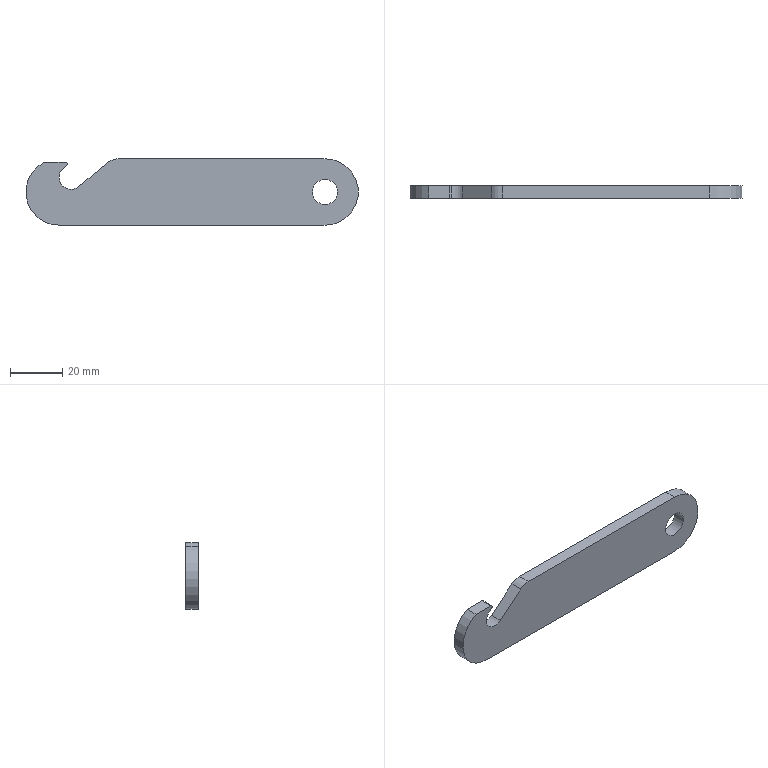Part | NX | features BREP 1 | 1 solid | 14 faces | box 127 x 4.763 x 25.4 mm | volume 13659 mm3 | plane 7 | cylinder 7 | commonest cylinder face diameters 9.55 x2 25.4 x2 1.524 x1 9.144 x1 12.7 x1
STEP:
#1=CARTESIAN_POINT('',(-28.191,0.,12.7));
#2=VERTEX_POINT('',#1);
#3=CARTESIAN_POINT('',(50.8,0.,12.7));
#4=VERTEX_POINT('',#3);
#5=CARTESIAN_POINT('',(-28.191,0.,12.7));
#6=DIRECTION('',(1.,0.,0.));
#7=VECTOR('',#6,1000.);
#8=LINE('',#5,#7);
#9=EDGE_CURVE('',#2,#4,#8,.T.);
#10=ORIENTED_EDGE('',*,*,#9,.T.);
#11=CARTESIAN_POINT('',(50.8,0.,-12.7));
#12=VERTEX_POINT('',#11);
#13=CARTESIAN_POINT('',(50.8,0.,0.));
#14=DIRECTION('',(0.,1.,0.));
#15=DIRECTION('',(0.,0.,1.));
#16=AXIS2_PLACEMENT_3D('',#13,#14,#15);
#17=CIRCLE('',#16,12.7);
#18=EDGE_CURVE('',#4,#12,#17,.T.);
#19=ORIENTED_EDGE('',*,*,#18,.T.);
#20=CARTESIAN_POINT('',(-50.8,0.,-12.7));
#21=VERTEX_POINT('',#20);
#22=CARTESIAN_POINT('',(50.8,0.,-12.7));
#23=DIRECTION('',(-1.,0.,0.));
#24=VECTOR('',#23,1000.);
#25=LINE('',#22,#24);
#26=EDGE_CURVE('',#12,#21,#25,.T.);
#27=ORIENTED_EDGE('',*,*,#26,.T.);
#28=CARTESIAN_POINT('',(-56.335,0.,11.43));
#29=VERTEX_POINT('',#28);
#30=CARTESIAN_POINT('',(-50.8,0.,0.));
#31=DIRECTION('',(0.,1.,0.));
#32=DIRECTION('',(0.,0.,-1.));
#33=AXIS2_PLACEMENT_3D('',#30,#31,#32);
#34=CIRCLE('',#33,12.7);
#35=EDGE_CURVE('',#21,#29,#34,.T.);
#36=ORIENTED_EDGE('',*,*,#35,.T.);
#37=CARTESIAN_POINT('',(-48.457,0.,11.43));
#38=VERTEX_POINT('',#37);
#39=CARTESIAN_POINT('',(-56.335,0.,11.43));
#40=CARTESIAN_POINT('',(-53.709,0.,11.43));
#41=CARTESIAN_POINT('',(-51.083,0.,11.43));
#42=CARTESIAN_POINT('',(-48.457,0.,11.43));
#43=B_SPLINE_CURVE_WITH_KNOTS('',3,(#39,#40,#41,#42),.UNSPECIFIED.,.F.,.F.,(4,4),(0.,1.),.UNSPECIFIED.);
#44=EDGE_CURVE('',#29,#38,#43,.T.);
#45=ORIENTED_EDGE('',*,*,#44,.T.);
#46=CARTESIAN_POINT('',(-47.971,0.,10.081));
#47=VERTEX_POINT('',#46);
#48=CARTESIAN_POINT('',(-48.457,0.,10.668));
#49=DIRECTION('',(0.,1.,0.));
#50=DIRECTION('',(0.,0.,1.));
#51=AXIS2_PLACEMENT_3D('',#48,#49,#50);
#52=CIRCLE('',#51,0.762);
#53=EDGE_CURVE('',#38,#47,#52,.T.);
#54=ORIENTED_EDGE('',*,*,#53,.T.);
#55=CARTESIAN_POINT('',(-49.145,0.,9.108));
#56=VERTEX_POINT('',#55);
#57=CARTESIAN_POINT('',(-47.971,0.,10.081));
#58=DIRECTION('',(-0.77,0.,-0.6381));
#59=VECTOR('',#58,1000.);
#60=LINE('',#57,#59);
#61=EDGE_CURVE('',#47,#56,#60,.T.);
#62=ORIENTED_EDGE('',*,*,#61,.T.);
#63=CARTESIAN_POINT('',(-43.311,0.,2.068));
#64=VERTEX_POINT('',#63);
#65=CARTESIAN_POINT('',(-46.228,0.,5.588));
#66=DIRECTION('',(0.,1.,0.));
#67=DIRECTION('',(0.6381,0.,-0.77));
#68=AXIS2_PLACEMENT_3D('',#65,#66,#67);
#69=CIRCLE('',#68,4.572);
#70=EDGE_CURVE('',#64,#56,#69,.T.);
#71=ORIENTED_EDGE('',*,*,#70,.F.);
#72=CARTESIAN_POINT('',(-32.243,0.,11.239));
#73=VERTEX_POINT('',#72);
#74=CARTESIAN_POINT('',(-43.311,0.,2.068));
#75=DIRECTION('',(0.77,0.,0.6381));
#76=VECTOR('',#75,1000.);
#77=LINE('',#74,#76);
#78=EDGE_CURVE('',#64,#73,#77,.T.);
#79=ORIENTED_EDGE('',*,*,#78,.T.);
#80=CARTESIAN_POINT('',(-28.191,0.,6.35));
#81=DIRECTION('',(0.,1.,0.));
#82=DIRECTION('',(-0.6381,0.,0.77));
#83=AXIS2_PLACEMENT_3D('',#80,#81,#82);
#84=CIRCLE('',#83,6.35);
#85=EDGE_CURVE('',#73,#2,#84,.T.);
#86=ORIENTED_EDGE('',*,*,#85,.T.);
#87=EDGE_LOOP('',(#10,#19,#27,#36,#45,#54,#62,#71,#79,#86));
#88=FACE_BOUND('',#87,.T.);
#89=CARTESIAN_POINT('',(55.575,0.,0.));
#90=VERTEX_POINT('',#89);
#91=CARTESIAN_POINT('',(46.025,0.,0.));
#92=VERTEX_POINT('',#91);
#93=CARTESIAN_POINT('',(50.8,0.,0.));
#94=DIRECTION('',(0.,1.,0.));
#95=DIRECTION('',(1.,0.,0.));
#96=AXIS2_PLACEMENT_3D('',#93,#94,#95);
#97=CIRCLE('',#96,4.775);
#98=EDGE_CURVE('',#90,#92,#97,.T.);
#99=ORIENTED_EDGE('',*,*,#98,.F.);
#100=CARTESIAN_POINT('',(50.8,0.,0.));
#101=DIRECTION('',(0.,1.,0.));
#102=DIRECTION('',(-1.,0.,0.));
#103=AXIS2_PLACEMENT_3D('',#100,#101,#102);
#104=CIRCLE('',#103,4.775);
#105=EDGE_CURVE('',#92,#90,#104,.T.);
#106=ORIENTED_EDGE('',*,*,#105,.F.);
#107=EDGE_LOOP('',(#99,#106));
#108=FACE_BOUND('',#107,.T.);
#109=CARTESIAN_POINT('',(0.,0.,0.));
#110=DIRECTION('',(0.,1.,0.));
#111=DIRECTION('',(1.,0.,0.));
#112=AXIS2_PLACEMENT_3D('',#109,#110,#111);
#113=PLANE('',#112);
#114=ADVANCED_FACE('',(#88,#108),#113,.T.);
#115=CARTESIAN_POINT('',(55.575,-4.763,0.));
#116=VERTEX_POINT('',#115);
#117=CARTESIAN_POINT('',(55.575,0.,0.));
#118=DIRECTION('',(0.,-1.,0.));
#119=VECTOR('',#118,1000.);
#120=LINE('',#117,#119);
#121=EDGE_CURVE('',#116,#90,#120,.F.);
#122=ORIENTED_EDGE('',*,*,#121,.F.);
#123=CARTESIAN_POINT('',(46.025,-4.763,0.));
#124=VERTEX_POINT('',#123);
#125=CARTESIAN_POINT('',(50.8,-4.763,0.));
#126=DIRECTION('',(0.,1.,0.));
#127=DIRECTION('',(-1.,0.,0.));
#128=AXIS2_PLACEMENT_3D('',#125,#126,#127);
#129=CIRCLE('',#128,4.775);
#130=EDGE_CURVE('',#124,#116,#129,.T.);
#131=ORIENTED_EDGE('',*,*,#130,.F.);
#132=CARTESIAN_POINT('',(46.025,0.,0.));
#133=DIRECTION('',(0.,-1.,0.));
#134=VECTOR('',#133,1000.);
#135=LINE('',#132,#134);
#136=EDGE_CURVE('',#124,#92,#135,.F.);
#137=ORIENTED_EDGE('',*,*,#136,.T.);
#138=ORIENTED_EDGE('',*,*,#105,.T.);
#139=EDGE_LOOP('',(#122,#131,#137,#138));
#140=FACE_BOUND('',#139,.T.);
#141=CARTESIAN_POINT('',(50.8,-2.381,0.));
#142=DIRECTION('',(0.,1.,0.));
#143=DIRECTION('',(-1.,0.,0.));
#144=AXIS2_PLACEMENT_3D('',#141,#142,#143);
#145=CYLINDRICAL_SURFACE('',#144,4.775);
#146=ADVANCED_FACE('',(#140),#145,.F.);
#147=ORIENTED_EDGE('',*,*,#136,.F.);
#148=CARTESIAN_POINT('',(50.8,-4.763,0.));
#149=DIRECTION('',(0.,1.,0.));
#150=DIRECTION('',(1.,0.,0.));
#151=AXIS2_PLACEMENT_3D('',#148,#149,#150);
#152=CIRCLE('',#151,4.775);
#153=EDGE_CURVE('',#116,#124,#152,.T.);
#154=ORIENTED_EDGE('',*,*,#153,.F.);
#155=ORIENTED_EDGE('',*,*,#121,.T.);
#156=ORIENTED_EDGE('',*,*,#98,.T.);
#157=EDGE_LOOP('',(#147,#154,#155,#156));
#158=FACE_BOUND('',#157,.T.);
#159=CARTESIAN_POINT('',(50.8,-2.381,0.));
#160=DIRECTION('',(0.,1.,0.));
#161=DIRECTION('',(1.,0.,0.));
#162=AXIS2_PLACEMENT_3D('',#159,#160,#161);
#163=CYLINDRICAL_SURFACE('',#162,4.775);
#164=ADVANCED_FACE('',(#158),#163,.F.);
#165=CARTESIAN_POINT('',(-43.311,-4.763,2.068));
#166=VERTEX_POINT('',#165);
#167=CARTESIAN_POINT('',(-32.243,-4.763,11.239));
#168=VERTEX_POINT('',#167);
#169=CARTESIAN_POINT('',(-43.311,-4.763,2.068));
#170=DIRECTION('',(0.77,0.,0.6381));
#171=VECTOR('',#170,1000.);
#172=LINE('',#169,#171);
#173=EDGE_CURVE('',#166,#168,#172,.T.);
#174=ORIENTED_EDGE('',*,*,#173,.F.);
#175=CARTESIAN_POINT('',(-49.145,-4.763,9.108));
#176=VERTEX_POINT('',#175);
#177=CARTESIAN_POINT('',(-46.228,-4.763,5.588));
#178=DIRECTION('',(0.,1.,0.));
#179=DIRECTION('',(0.6381,0.,-0.77));
#180=AXIS2_PLACEMENT_3D('',#177,#178,#179);
#181=CIRCLE('',#180,4.572);
#182=EDGE_CURVE('',#166,#176,#181,.T.);
#183=ORIENTED_EDGE('',*,*,#182,.T.);
#184=CARTESIAN_POINT('',(-47.971,-4.763,10.081));
#185=VERTEX_POINT('',#184);
#186=CARTESIAN_POINT('',(-47.971,-4.763,10.081));
#187=DIRECTION('',(-0.77,0.,-0.6381));
#188=VECTOR('',#187,1000.);
#189=LINE('',#186,#188);
#190=EDGE_CURVE('',#185,#176,#189,.T.);
#191=ORIENTED_EDGE('',*,*,#190,.F.);
#192=CARTESIAN_POINT('',(-48.457,-4.763,11.43));
#193=VERTEX_POINT('',#192);
#194=CARTESIAN_POINT('',(-48.457,-4.763,10.668));
#195=DIRECTION('',(0.,1.,0.));
#196=DIRECTION('',(0.,0.,1.));
#197=AXIS2_PLACEMENT_3D('',#194,#195,#196);
#198=CIRCLE('',#197,0.762);
#199=EDGE_CURVE('',#193,#185,#198,.T.);
#200=ORIENTED_EDGE('',*,*,#199,.F.);
#201=CARTESIAN_POINT('',(-56.335,-4.763,11.43));
#202=VERTEX_POINT('',#201);
#203=CARTESIAN_POINT('',(-48.457,-4.763,11.43));
#204=CARTESIAN_POINT('',(-51.083,-4.763,11.43));
#205=CARTESIAN_POINT('',(-53.709,-4.763,11.43));
#206=CARTESIAN_POINT('',(-56.335,-4.763,11.43));
#207=B_SPLINE_CURVE_WITH_KNOTS('',3,(#203,#204,#205,#206),.UNSPECIFIED.,.F.,.F.,(4,4),(0.,1.),.UNSPECIFIED.);
#208=EDGE_CURVE('',#202,#193,#207,.F.);
#209=ORIENTED_EDGE('',*,*,#208,.F.);
#210=CARTESIAN_POINT('',(-50.8,-4.763,-12.7));
#211=VERTEX_POINT('',#210);
#212=CARTESIAN_POINT('',(-50.8,-4.763,0.));
#213=DIRECTION('',(0.,1.,0.));
#214=DIRECTION('',(0.,0.,-1.));
#215=AXIS2_PLACEMENT_3D('',#212,#213,#214);
#216=CIRCLE('',#215,12.7);
#217=EDGE_CURVE('',#211,#202,#216,.T.);
#218=ORIENTED_EDGE('',*,*,#217,.F.);
#219=CARTESIAN_POINT('',(50.8,-4.763,-12.7));
#220=VERTEX_POINT('',#219);
#221=CARTESIAN_POINT('',(50.8,-4.763,-12.7));
#222=DIRECTION('',(-1.,0.,0.));
#223=VECTOR('',#222,1000.);
#224=LINE('',#221,#223);
#225=EDGE_CURVE('',#220,#211,#224,.T.);
#226=ORIENTED_EDGE('',*,*,#225,.F.);
#227=CARTESIAN_POINT('',(50.8,-4.763,12.7));
#228=VERTEX_POINT('',#227);
#229=CARTESIAN_POINT('',(50.8,-4.763,0.));
#230=DIRECTION('',(0.,1.,0.));
#231=DIRECTION('',(0.,0.,1.));
#232=AXIS2_PLACEMENT_3D('',#229,#230,#231);
#233=CIRCLE('',#232,12.7);
#234=EDGE_CURVE('',#228,#220,#233,.T.);
#235=ORIENTED_EDGE('',*,*,#234,.F.);
#236=CARTESIAN_POINT('',(-28.191,-4.763,12.7));
#237=VERTEX_POINT('',#236);
#238=CARTESIAN_POINT('',(-28.191,-4.763,12.7));
#239=DIRECTION('',(1.,0.,0.));
#240=VECTOR('',#239,1000.);
#241=LINE('',#238,#240);
#242=EDGE_CURVE('',#237,#228,#241,.T.);
#243=ORIENTED_EDGE('',*,*,#242,.F.);
#244=CARTESIAN_POINT('',(-28.191,-4.763,6.35));
#245=DIRECTION('',(0.,-1.,0.));
#246=DIRECTION('',(0.,0.,1.));
#247=AXIS2_PLACEMENT_3D('',#244,#245,#246);
#248=CIRCLE('',#247,6.35);
#249=EDGE_CURVE('',#237,#168,#248,.T.);
#250=ORIENTED_EDGE('',*,*,#249,.T.);
#251=EDGE_LOOP('',(#174,#183,#191,#200,#209,#218,#226,#235,#243,#250));
#252=FACE_BOUND('',#251,.T.);
#253=ORIENTED_EDGE('',*,*,#153,.T.);
#254=ORIENTED_EDGE('',*,*,#130,.T.);
#255=EDGE_LOOP('',(#253,#254));
#256=FACE_BOUND('',#255,.T.);
#257=CARTESIAN_POINT('',(0.,-4.763,0.));
#258=DIRECTION('',(0.,1.,0.));
#259=DIRECTION('',(1.,0.,0.));
#260=AXIS2_PLACEMENT_3D('',#257,#258,#259);
#261=PLANE('',#260);
#262=ADVANCED_FACE('',(#252,#256),#261,.F.);
#263=ORIENTED_EDGE('',*,*,#249,.F.);
#264=CARTESIAN_POINT('',(-28.191,-4.763,12.7));
#265=DIRECTION('',(0.,1.,0.));
#266=VECTOR('',#265,1000.);
#267=LINE('',#264,#266);
#268=EDGE_CURVE('',#237,#2,#267,.T.);
#269=ORIENTED_EDGE('',*,*,#268,.T.);
#270=ORIENTED_EDGE('',*,*,#85,.F.);
#271=CARTESIAN_POINT('',(-32.243,-4.763,11.239));
#272=DIRECTION('',(0.,1.,0.));
#273=VECTOR('',#272,1000.);
#274=LINE('',#271,#273);
#275=EDGE_CURVE('',#168,#73,#274,.T.);
#276=ORIENTED_EDGE('',*,*,#275,.F.);
#277=EDGE_LOOP('',(#263,#269,#270,#276));
#278=FACE_BOUND('',#277,.T.);
#279=CARTESIAN_POINT('',(-28.191,-4.953,6.35));
#280=DIRECTION('',(0.,1.,0.));
#281=DIRECTION('',(-0.6381,0.,0.77));
#282=AXIS2_PLACEMENT_3D('',#279,#280,#281);
#283=CYLINDRICAL_SURFACE('',#282,6.35);
#284=ADVANCED_FACE('',(#278),#283,.T.);
#285=ORIENTED_EDGE('',*,*,#78,.F.);
#286=CARTESIAN_POINT('',(-43.311,0.,2.068));
#287=DIRECTION('',(0.,-1.,0.));
#288=VECTOR('',#287,1000.);
#289=LINE('',#286,#288);
#290=EDGE_CURVE('',#64,#166,#289,.T.);
#291=ORIENTED_EDGE('',*,*,#290,.T.);
#292=ORIENTED_EDGE('',*,*,#173,.T.);
#293=ORIENTED_EDGE('',*,*,#275,.T.);
#294=EDGE_LOOP('',(#285,#291,#292,#293));
#295=FACE_BOUND('',#294,.T.);
#296=CARTESIAN_POINT('',(-36.895,-2.381,7.384));
#297=DIRECTION('',(-0.6381,0.,0.77));
#298=DIRECTION('',(0.,1.,0.));
#299=AXIS2_PLACEMENT_3D('',#296,#297,#298);
#300=PLANE('',#299);
#301=ADVANCED_FACE('',(#295),#300,.T.);
#302=CARTESIAN_POINT('',(-49.145,0.,9.108));
#303=DIRECTION('',(0.,-1.,0.));
#304=VECTOR('',#303,1000.);
#305=LINE('',#302,#304);
#306=EDGE_CURVE('',#56,#176,#305,.T.);
#307=ORIENTED_EDGE('',*,*,#306,.T.);
#308=ORIENTED_EDGE('',*,*,#182,.F.);
#309=ORIENTED_EDGE('',*,*,#290,.F.);
#310=ORIENTED_EDGE('',*,*,#70,.T.);
#311=EDGE_LOOP('',(#307,#308,#309,#310));
#312=FACE_BOUND('',#311,.T.);
#313=CARTESIAN_POINT('',(-46.228,-2.381,5.588));
#314=DIRECTION('',(0.,1.,0.));
#315=DIRECTION('',(0.6381,0.,-0.77));
#316=AXIS2_PLACEMENT_3D('',#313,#314,#315);
#317=CYLINDRICAL_SURFACE('',#316,4.572);
#318=ADVANCED_FACE('',(#312),#317,.F.);
#319=CARTESIAN_POINT('',(-47.971,0.,10.081));
#320=DIRECTION('',(0.,-1.,0.));
#321=VECTOR('',#320,1000.);
#322=LINE('',#319,#321);
#323=EDGE_CURVE('',#47,#185,#322,.T.);
#324=ORIENTED_EDGE('',*,*,#323,.T.);
#325=ORIENTED_EDGE('',*,*,#190,.T.);
#326=ORIENTED_EDGE('',*,*,#306,.F.);
#327=ORIENTED_EDGE('',*,*,#61,.F.);
#328=EDGE_LOOP('',(#324,#325,#326,#327));
#329=FACE_BOUND('',#328,.T.);
#330=CARTESIAN_POINT('',(-48.558,-2.381,9.595));
#331=DIRECTION('',(0.6381,0.,-0.77));
#332=DIRECTION('',(0.,-1.,0.));
#333=AXIS2_PLACEMENT_3D('',#330,#331,#332);
#334=PLANE('',#333);
#335=ADVANCED_FACE('',(#329),#334,.T.);
#336=CARTESIAN_POINT('',(-48.457,0.,11.43));
#337=DIRECTION('',(0.,-1.,0.));
#338=VECTOR('',#337,1000.);
#339=LINE('',#336,#338);
#340=EDGE_CURVE('',#38,#193,#339,.T.);
#341=ORIENTED_EDGE('',*,*,#340,.T.);
#342=ORIENTED_EDGE('',*,*,#199,.T.);
#343=ORIENTED_EDGE('',*,*,#323,.F.);
#344=ORIENTED_EDGE('',*,*,#53,.F.);
#345=EDGE_LOOP('',(#341,#342,#343,#344));
#346=FACE_BOUND('',#345,.T.);
#347=CARTESIAN_POINT('',(-48.457,-2.381,10.668));
#348=DIRECTION('',(0.,1.,0.));
#349=DIRECTION('',(0.,0.,1.));
#350=AXIS2_PLACEMENT_3D('',#347,#348,#349);
#351=CYLINDRICAL_SURFACE('',#350,0.762);
#352=ADVANCED_FACE('',(#346),#351,.T.);
#353=CARTESIAN_POINT('',(-56.335,0.,11.43));
#354=CARTESIAN_POINT('',(-56.335,-1.587,11.43));
#355=CARTESIAN_POINT('',(-56.335,-3.175,11.43));
#356=CARTESIAN_POINT('',(-56.335,-4.763,11.43));
#357=B_SPLINE_CURVE_WITH_KNOTS('',3,(#353,#354,#355,#356),.UNSPECIFIED.,.F.,.F.,(4,4),(0.,1.),.UNSPECIFIED.);
#358=EDGE_CURVE('',#29,#202,#357,.T.);
#359=ORIENTED_EDGE('',*,*,#358,.T.);
#360=ORIENTED_EDGE('',*,*,#208,.T.);
#361=ORIENTED_EDGE('',*,*,#340,.F.);
#362=ORIENTED_EDGE('',*,*,#44,.F.);
#363=EDGE_LOOP('',(#359,#360,#361,#362));
#364=FACE_BOUND('',#363,.T.);
#365=CARTESIAN_POINT('',(-52.396,-2.381,11.43));
#366=DIRECTION('',(0.,0.,1.));
#367=DIRECTION('',(1.,0.,0.));
#368=AXIS2_PLACEMENT_3D('',#365,#366,#367);
#369=PLANE('',#368);
#370=ADVANCED_FACE('',(#364),#369,.T.);
#371=ORIENTED_EDGE('',*,*,#35,.F.);
#372=CARTESIAN_POINT('',(-50.8,0.,-12.7));
#373=DIRECTION('',(0.,-1.,0.));
#374=VECTOR('',#373,1000.);
#375=LINE('',#372,#374);
#376=EDGE_CURVE('',#21,#211,#375,.T.);
#377=ORIENTED_EDGE('',*,*,#376,.T.);
#378=ORIENTED_EDGE('',*,*,#217,.T.);
#379=ORIENTED_EDGE('',*,*,#358,.F.);
#380=EDGE_LOOP('',(#371,#377,#378,#379));
#381=FACE_BOUND('',#380,.T.);
#382=CARTESIAN_POINT('',(-50.8,-2.381,0.));
#383=DIRECTION('',(0.,1.,0.));
#384=DIRECTION('',(0.,0.,-1.));
#385=AXIS2_PLACEMENT_3D('',#382,#383,#384);
#386=CYLINDRICAL_SURFACE('',#385,12.7);
#387=ADVANCED_FACE('',(#381),#386,.T.);
#388=CARTESIAN_POINT('',(50.8,0.,-12.7));
#389=DIRECTION('',(0.,-1.,0.));
#390=VECTOR('',#389,1000.);
#391=LINE('',#388,#390);
#392=EDGE_CURVE('',#12,#220,#391,.T.);
#393=ORIENTED_EDGE('',*,*,#392,.T.);
#394=ORIENTED_EDGE('',*,*,#225,.T.);
#395=ORIENTED_EDGE('',*,*,#376,.F.);
#396=ORIENTED_EDGE('',*,*,#26,.F.);
#397=EDGE_LOOP('',(#393,#394,#395,#396));
#398=FACE_BOUND('',#397,.T.);
#399=CARTESIAN_POINT('',(0.,-2.381,-12.7));
#400=DIRECTION('',(0.,0.,-1.));
#401=DIRECTION('',(0.,-1.,0.));
#402=AXIS2_PLACEMENT_3D('',#399,#400,#401);
#403=PLANE('',#402);
#404=ADVANCED_FACE('',(#398),#403,.T.);
#405=CARTESIAN_POINT('',(50.8,0.,12.7));
#406=DIRECTION('',(0.,-1.,0.));
#407=VECTOR('',#406,1000.);
#408=LINE('',#405,#407);
#409=EDGE_CURVE('',#4,#228,#408,.T.);
#410=ORIENTED_EDGE('',*,*,#409,.T.);
#411=ORIENTED_EDGE('',*,*,#234,.T.);
#412=ORIENTED_EDGE('',*,*,#392,.F.);
#413=ORIENTED_EDGE('',*,*,#18,.F.);
#414=EDGE_LOOP('',(#410,#411,#412,#413));
#415=FACE_BOUND('',#414,.T.);
#416=CARTESIAN_POINT('',(50.8,-2.381,0.));
#417=DIRECTION('',(0.,1.,0.));
#418=DIRECTION('',(0.,0.,1.));
#419=AXIS2_PLACEMENT_3D('',#416,#417,#418);
#420=CYLINDRICAL_SURFACE('',#419,12.7);
#421=ADVANCED_FACE('',(#415),#420,.T.);
#422=ORIENTED_EDGE('',*,*,#242,.T.);
#423=ORIENTED_EDGE('',*,*,#409,.F.);
#424=ORIENTED_EDGE('',*,*,#9,.F.);
#425=ORIENTED_EDGE('',*,*,#268,.F.);
#426=EDGE_LOOP('',(#422,#423,#424,#425));
#427=FACE_BOUND('',#426,.T.);
#428=CARTESIAN_POINT('',(0.,-2.381,12.7));
#429=DIRECTION('',(0.,0.,1.));
#430=DIRECTION('',(1.,0.,0.));
#431=AXIS2_PLACEMENT_3D('',#428,#429,#430);
#432=PLANE('',#431);
#433=ADVANCED_FACE('',(#427),#432,.T.);
#434=CLOSED_SHELL('',(#114,#146,#164,#262,#284,#301,#318,#335,#352,#370,#387,#404,#421,#433));
#435=MANIFOLD_SOLID_BREP('',#434);
#436=(LENGTH_UNIT()NAMED_UNIT(*)SI_UNIT(.MILLI.,.METRE.));
#437=UNCERTAINTY_MEASURE_WITH_UNIT(LENGTH_MEASURE(0.0508),#436,'','');
#438=(NAMED_UNIT(*)PLANE_ANGLE_UNIT()SI_UNIT($,.RADIAN.));
#439=(NAMED_UNIT(*)SI_UNIT($,.STERADIAN.)SOLID_ANGLE_UNIT());
#440=(GEOMETRIC_REPRESENTATION_CONTEXT(3)GLOBAL_UNCERTAINTY_ASSIGNED_CONTEXT((#437))GLOBAL_UNIT_ASSIGNED_CONTEXT((#436,#438,#439))REPRESENTATION_CONTEXT('',''));
#441=ADVANCED_BREP_SHAPE_REPRESENTATION('',(#435),#440);